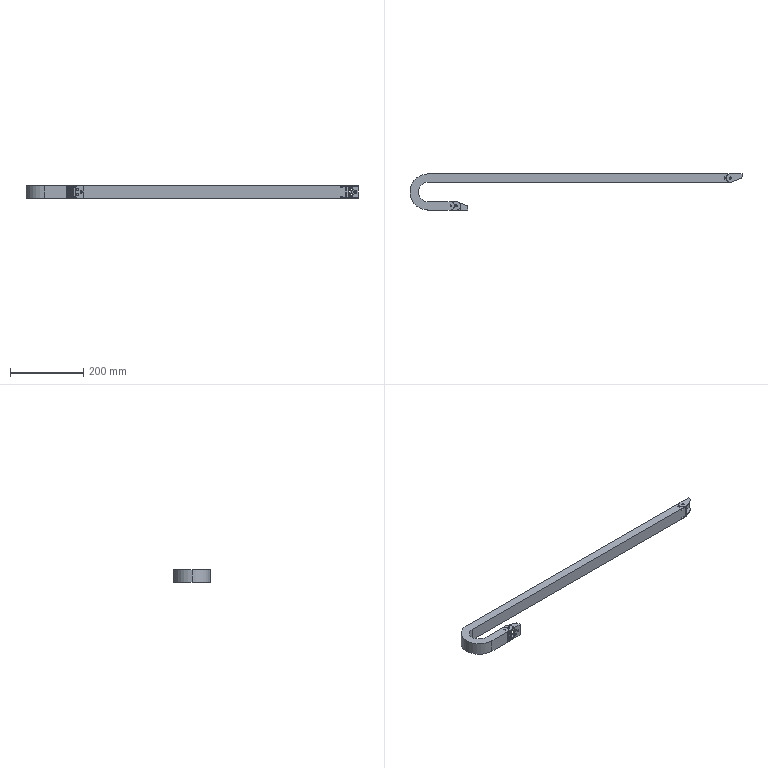Part | SolidWorks | features MoveCopyBody 4, ICE 3, Split 2, BaseBody 1 | 1 solid | 258 faces | box 907.2 x 99 x 35 mm | volume 815735 mm3 | plane 165 | cylinder 66 | cone 17 | spline 10 | commonest cylinder face diameters 5.2 x15 6 x12 25.4 x12 23 x8 10 x4 23.4 x4